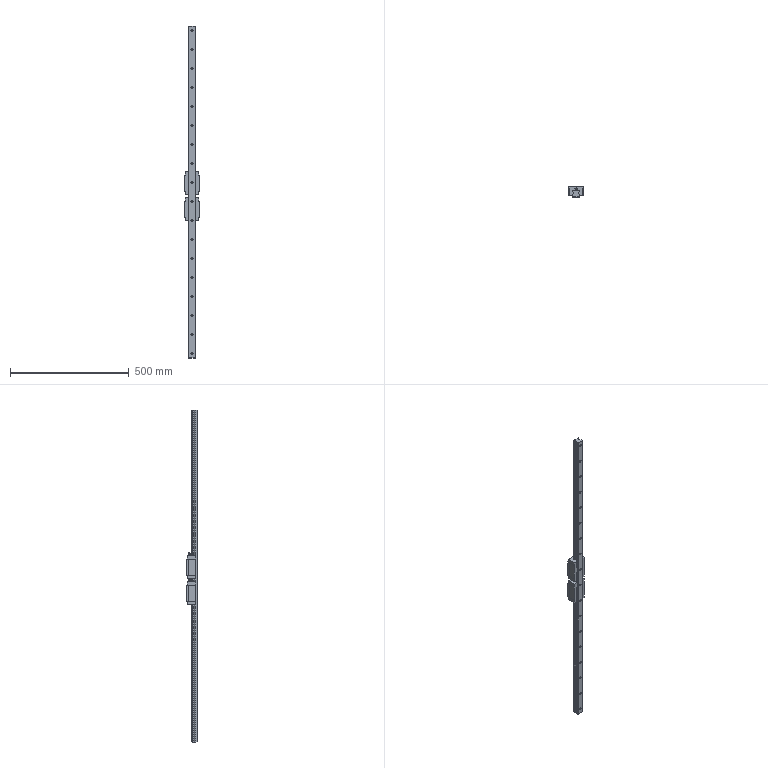Part | SolidWorks | 3 solids | 390 faces | box 60 x 45 x 1400 mm | volume 1198347 mm3 | plane 202 | cylinder 134 | cone 52 | sphere 2 | commonest cylinder face diameters 9 x36 14 x36 8 x16 1.152 x10 1.613 x8 7.2 x8